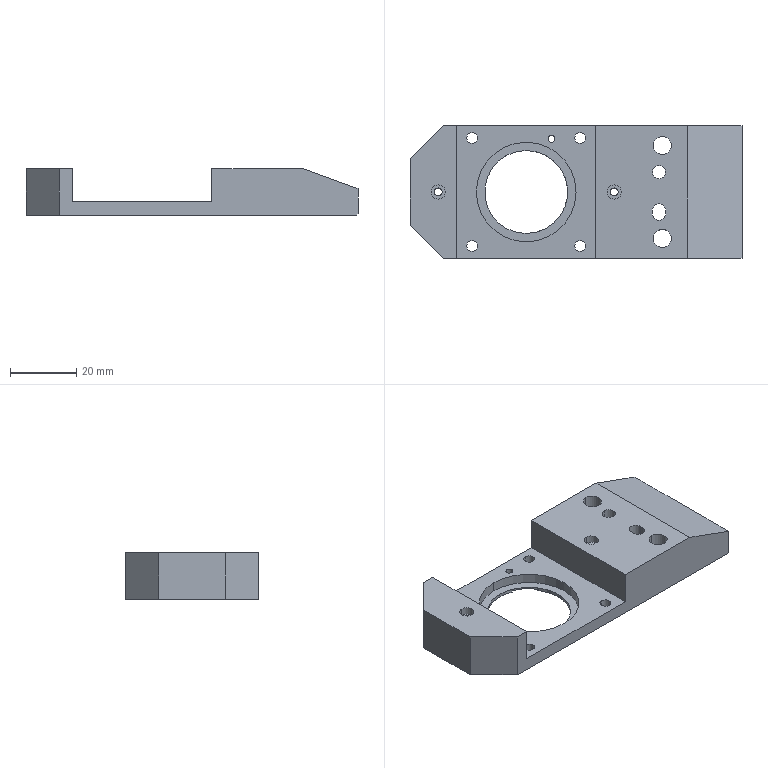NC program | NX | posted with a generic post | part box 100 x 40 x 14 mm
Lines 8469 to 9279 of 15435:
(HOLE_MILLING , TOOL : D3)
N16852 T17 M6
N16854 G54
N16856 G17 G0 G90 X-41.5 Y0. S5500 M3
N16858 G43 Z30. H17
N16860 Z0.5
N16862 G94 G3 X-41.175 Y-0.325 R0.325 F1250.
N16864 X-40.85 Y0. R0.325
N16866 X-40.85 Y0. Z0.44 I-0.65 J0.
N16868 X-40.85 Y0. Z0.38 I-0.65 J0.
N16870 X-40.85 Y0. Z0.32 I-0.65 J0.
N16872 X-40.85 Y0. Z0.26 I-0.65 J0.
N16874 X-40.85 Y0. Z0.2 I-0.65 J0.
N16876 X-40.85 Y0. Z0.14 I-0.65 J0.
N16878 X-40.85 Y0. Z0.08 I-0.65 J0.
N16880 X-40.85 Y0. Z0.02 I-0.65 J0.
N16882 X-40.85 Y0. Z-0.04 I-0.65 J0.
N16884 X-40.85 Y0. Z-0.1 I-0.65 J0.
N16886 X-40.85 Y0. Z-0.16 I-0.65 J0.
N16888 X-40.85 Y0. Z-0.22 I-0.65 J0.
N16890 X-40.85 Y0. Z-0.28 I-0.65 J0.
N16892 X-40.85 Y0. Z-0.34 I-0.65 J0.
N16894 X-40.85 Y0. Z-0.4 I-0.65 J0.
N16896 X-40.85 Y0. Z-0.46 I-0.65 J0.
N16898 X-40.85 Y0. Z-0.52 I-0.65 J0.
N16900 X-40.85 Y0. Z-0.58 I-0.65 J0.
N16902 X-40.85 Y0. Z-0.64 I-0.65 J0.
N16904 X-40.85 Y0. Z-0.7 I-0.65 J0.
N16906 X-40.85 Y0. Z-0.76 I-0.65 J0.
N16908 X-40.85 Y0. Z-0.82 I-0.65 J0.
N16910 X-40.85 Y0. Z-0.88 I-0.65 J0.
N16912 X-40.85 Y0. Z-0.94 I-0.65 J0.
N16914 X-40.85 Y0. Z-1. I-0.65 J0.
N16916 X-40.85 Y0. Z-1.06 I-0.65 J0.
N16918 X-40.85 Y0. Z-1.12 I-0.65 J0.
N16920 X-40.85 Y0. Z-1.18 I-0.65 J0.
N16922 X-40.85 Y0. Z-1.24 I-0.65 J0.
N16924 X-40.85 Y0. Z-1.3 I-0.65 J0.
N16926 X-40.85 Y0. Z-1.36 I-0.65 J0.
N16928 X-40.85 Y0. Z-1.42 I-0.65 J0.
N16930 X-40.85 Y0. Z-1.48 I-0.65 J0.
N16932 X-40.85 Y0. Z-1.54 I-0.65 J0.
N16934 X-40.85 Y0. Z-1.6 I-0.65 J0.
N16936 X-40.85 Y0. Z-1.66 I-0.65 J0.
N16938 X-40.85 Y0. Z-1.72 I-0.65 J0.
N16940 X-40.85 Y0. Z-1.78 I-0.65 J0.
N16942 X-40.85 Y0. Z-1.84 I-0.65 J0.
N16944 X-40.85 Y0. Z-1.9 I-0.65 J0.
N16946 X-40.85 Y0. Z-1.96 I-0.65 J0.
N16948 X-40.85 Y0. Z-2.02 I-0.65 J0.
N16950 X-40.85 Y0. Z-2.08 I-0.65 J0.
N16952 X-40.85 Y0. Z-2.14 I-0.65 J0.
N16954 X-40.85 Y0. Z-2.2 I-0.65 J0.
N16956 X-40.85 Y0. Z-2.26 I-0.65 J0.
N16958 X-41.825 Y-0.563 Z-2.3 R-0.65
N16960 X-40.937 Y-0.325 R0.65
N16962 X-41.825 Y-0.563 R-0.65
N16964 X-41.381 Y-0.444 R0.325
N16966 X-41.5 Y0. R0.325
N16968 G0 Z30.
N16970 X11.5
N16972 Z0.5
N16974 G3 X11.825 Y-0.325 R0.325
N16976 X12.15 Y0. R0.325
N16978 X12.15 Y0. Z0.44 I-0.65 J0.
N16980 X12.15 Y0. Z0.38 I-0.65 J0.
N16982 X12.15 Y0. Z0.32 I-0.65 J0.
N16984 X12.15 Y0. Z0.26 I-0.65 J0.
N16986 X12.15 Y0. Z0.2 I-0.65 J0.
N16988 X12.15 Y0. Z0.14 I-0.65 J0.
N16990 X12.15 Y0. Z0.08 I-0.65 J0.
N16992 X12.15 Y0. Z0.02 I-0.65 J0.
N16994 X12.15 Y0. Z-0.04 I-0.65 J0.
N16996 X12.15 Y0. Z-0.1 I-0.65 J0.
N16998 X12.15 Y0. Z-0.16 I-0.65 J0.
N17000 X12.15 Y0. Z-0.22 I-0.65 J0.
N17002 X12.15 Y0. Z-0.28 I-0.65 J0.
N17004 X12.15 Y0. Z-0.34 I-0.65 J0.
N17006 X12.15 Y0. Z-0.4 I-0.65 J0.
N17008 X12.15 Y0. Z-0.46 I-0.65 J0.
N17010 X12.15 Y0. Z-0.52 I-0.65 J0.
N17012 X12.15 Y0. Z-0.58 I-0.65 J0.
N17014 X12.15 Y0. Z-0.64 I-0.65 J0.
N17016 X12.15 Y0. Z-0.7 I-0.65 J0.
N17018 X12.15 Y0. Z-0.76 I-0.65 J0.
N17020 X12.15 Y0. Z-0.82 I-0.65 J0.
N17022 X12.15 Y0. Z-0.88 I-0.65 J0.
N17024 X12.15 Y0. Z-0.94 I-0.65 J0.
N17026 X12.15 Y0. Z-1. I-0.65 J0.
N17028 X12.15 Y0. Z-1.06 I-0.65 J0.
N17030 X12.15 Y0. Z-1.12 I-0.65 J0.
N17032 X12.15 Y0. Z-1.18 I-0.65 J0.
N17034 X12.15 Y0. Z-1.24 I-0.65 J0.
N17036 X12.15 Y0. Z-1.3 I-0.65 J0.
N17038 X12.15 Y0. Z-1.36 I-0.65 J0.
N17040 X12.15 Y0. Z-1.42 I-0.65 J0.
N17042 X12.15 Y0. Z-1.48 I-0.65 J0.
N17044 X12.15 Y0. Z-1.54 I-0.65 J0.
N17046 X12.15 Y0. Z-1.6 I-0.65 J0.
N17048 X12.15 Y0. Z-1.66 I-0.65 J0.
N17050 X12.15 Y0. Z-1.72 I-0.65 J0.
N17052 X12.15 Y0. Z-1.78 I-0.65 J0.
N17054 X12.15 Y0. Z-1.84 I-0.65 J0.
N17056 X12.15 Y0. Z-1.9 I-0.65 J0.
N17058 X12.15 Y0. Z-1.96 I-0.65 J0.
N17060 X12.15 Y0. Z-2.02 I-0.65 J0.
N17062 X12.15 Y0. Z-2.08 I-0.65 J0.
N17064 X12.15 Y0. Z-2.14 I-0.65 J0.
N17066 X12.15 Y0. Z-2.2 I-0.65 J0.
N17068 X12.15 Y0. Z-2.26 I-0.65 J0.
N17070 X11.175 Y-0.563 Z-2.3 R-0.65
N17072 X12.063 Y-0.325 R0.65
N17074 X11.175 Y-0.563 R-0.65
N17076 X11.619 Y-0.444 R0.325
N17078 X11.5 Y0. R0.325
N17080 G0 Z30.
(ZLEVEL_PROFILE_COPY_COPY_COPY , TOOL : D3)
N17082 X25.068 Y-5.056 S4500
N17084 Z1.
N17086 G1 X24.882 Z0.99 F1000.
N17088 X24.676 Y-5.173 Z0.978
N17090 X24.571 Y-5.333 Z0.968
N17092 X24.55 Y-5.405 Z0.964
N17094 Y-6.595 Z0.901
N17096 X24.676 Y-6.827 Z0.888
N17098 X24.908 Y-6.951 Z0.874
N17100 X25.099 Y-6.949 Z0.864
N17102 X25.327 Y-6.824 Z0.85
N17104 X25.45 Y-6.595 Z0.837
N17106 Y-5.405 Z0.774
N17108 X25.429 Y-5.333 Z0.77
N17110 X25.324 Y-5.173 Z0.76
N17112 X25.118 Y-5.056 Z0.748
N17114 X24.882 Z0.736
N17116 X24.676 Y-5.173 Z0.723
N17118 X24.571 Y-5.333 Z0.713
N17120 X24.55 Y-5.405 Z0.709
N17122 Y-6.595 Z0.647
N17124 X24.676 Y-6.827 Z0.633
N17126 X24.908 Y-6.951 Z0.619
N17128 X25.099 Y-6.949 Z0.609
N17130 X25.327 Y-6.824 Z0.596
N17132 X25.45 Y-6.595 Z0.582
N17134 Y-5.405 Z0.52
N17136 X25.429 Y-5.333 Z0.516
N17138 X25.324 Y-5.173 Z0.506
N17140 X25.118 Y-5.056 Z0.493
N17142 X24.882 Z0.481
N17144 X24.676 Y-5.173 Z0.468
N17146 X24.571 Y-5.333 Z0.458
N17148 X24.55 Y-5.405 Z0.454
N17150 Y-6.595 Z0.392
N17152 X24.676 Y-6.827 Z0.378
N17154 X24.908 Y-6.951 Z0.364
N17156 X25.099 Y-6.949 Z0.354
N17158 X25.327 Y-6.824 Z0.341
N17160 X25.45 Y-6.595 Z0.327
N17162 Y-5.405 Z0.265
N17164 X25.429 Y-5.333 Z0.261
N17166 X25.324 Y-5.173 Z0.251
N17168 X25.118 Y-5.056 Z0.238
N17170 X24.882 Z0.226
N17172 X24.676 Y-5.173 Z0.214
N17174 X24.571 Y-5.333 Z0.204
N17176 X24.55 Y-5.405 Z0.2
N17178 Y-6.595 Z0.137
N17180 X24.676 Y-6.827 Z0.124
N17182 X24.908 Y-6.951 Z0.11
N17184 X25.099 Y-6.949 Z0.1
N17186 X25.327 Y-6.824 Z0.086
N17188 X25.45 Y-6.595 Z0.072
N17190 Y-5.405 Z0.01
N17192 X25.429 Y-5.333 Z0.006
N17194 X25.324 Y-5.173 Z-0.004
N17196 X25.118 Y-5.056 Z-0.016
N17198 X24.882 Z-0.029
N17200 X24.676 Y-5.173 Z-0.041
N17202 X24.571 Y-5.333 Z-0.051
N17204 X24.55 Y-5.405 Z-0.055
N17206 Y-5.5 Z-0.06
N17208 Y-6.5 F1200.
N17210 G3 X25. Y-6.95 R0.45
N17212 X25.45 Y-6.5 R0.45
N17214 G1 Y-5.5
N17216 G3 X25. Y-5.05 R0.45
N17218 X24.55 Y-5.5 R0.45
N17220 G1 Y-6.482 Z-0.077
N17222 X24.565 Y-6.588 Z-0.079
N17224 X24.577 Y-6.639 Z-0.08
N17226 X24.588 Y-6.665
N17228 X24.613 Y-6.714 Z-0.081
N17230 X24.674 Y-6.798 Z-0.083
N17232 X24.732 Y-6.851 Z-0.085
N17234 X24.781 Y-6.884 Z-0.086
N17236 X24.871 Y-6.923 Z-0.087
N17238 X24.918 Y-6.934 Z-0.088
N17240 X24.949 Y-6.938 Z-0.089
N17242 X25.012 Y-6.942 Z-0.09
N17244 X25.108 Y-6.929 Z-0.092
N17246 X25.153 Y-6.915 Z-0.093
N17248 X25.183 Y-6.903
N17250 X25.239 Y-6.872 Z-0.094
N17252 X25.317 Y-6.811 Z-0.096
N17254 X25.366 Y-6.749 Z-0.097
N17256 X25.398 Y-6.694 Z-0.099
N17258 X25.421 Y-6.633 Z-0.1
N17260 X25.431 Y-6.602
N17262 X25.437 Y-6.554 Z-0.101
N17264 X25.448 Y-6.458 Z-0.103
N17266 X25.45 Y-6.336 Z-0.105
N17268 Y-5.722 Z-0.116
N17270 Y-5.599 Z-0.118
N17272 X25.449 Y-5.476 Z-0.12
N17274 G3 X24.55 Y-5.5 R0.45
N17276 G1 Y-6.482 Z-0.137
N17278 X24.565 Y-6.588 Z-0.139
N17280 X24.577 Y-6.639 Z-0.14
N17282 X24.588 Y-6.665
N17284 X24.613 Y-6.714 Z-0.141
N17286 X24.674 Y-6.798 Z-0.143
N17288 X24.732 Y-6.851 Z-0.145
N17290 X24.781 Y-6.884 Z-0.146
N17292 X24.871 Y-6.923 Z-0.147
N17294 X24.918 Y-6.934 Z-0.148
N17296 X24.949 Y-6.938 Z-0.149
N17298 X25.012 Y-6.942 Z-0.15
N17300 X25.108 Y-6.929 Z-0.152
N17302 X25.153 Y-6.915 Z-0.153
N17304 X25.183 Y-6.903
N17306 X25.239 Y-6.872 Z-0.154
N17308 X25.317 Y-6.811 Z-0.156
N17310 X25.366 Y-6.749 Z-0.157
N17312 X25.398 Y-6.694 Z-0.159
N17314 X25.421 Y-6.633 Z-0.16
N17316 X25.431 Y-6.602
N17318 X25.437 Y-6.554 Z-0.161
N17320 X25.448 Y-6.458 Z-0.163
N17322 X25.45 Y-6.336 Z-0.165
N17324 Y-5.722 Z-0.176
N17326 Y-5.599 Z-0.178
N17328 X25.449 Y-5.476 Z-0.18
N17330 G3 X24.55 Y-5.5 R0.45
N17332 G1 Y-6.482 Z-0.197
N17334 X24.565 Y-6.588 Z-0.199
N17336 X24.577 Y-6.639 Z-0.2
N17338 X24.588 Y-6.665
N17340 X24.613 Y-6.714 Z-0.201
N17342 X24.674 Y-6.798 Z-0.203
N17344 X24.732 Y-6.851 Z-0.205
N17346 X24.781 Y-6.884 Z-0.206
N17348 X24.871 Y-6.923 Z-0.207
N17350 X24.918 Y-6.934 Z-0.208
N17352 X24.949 Y-6.938 Z-0.209
N17354 X25.012 Y-6.942 Z-0.21
N17356 X25.108 Y-6.929 Z-0.212
N17358 X25.153 Y-6.915 Z-0.213
N17360 X25.183 Y-6.903
N17362 X25.239 Y-6.872 Z-0.214
N17364 X25.317 Y-6.811 Z-0.216
N17366 X25.366 Y-6.749 Z-0.217
N17368 X25.398 Y-6.694 Z-0.219
N17370 X25.421 Y-6.633 Z-0.22
N17372 X25.431 Y-6.602
N17374 X25.437 Y-6.554 Z-0.221
N17376 X25.448 Y-6.458 Z-0.223
N17378 X25.45 Y-6.336 Z-0.225
N17380 Y-5.722 Z-0.236
N17382 Y-5.599 Z-0.238
N17384 X25.449 Y-5.476 Z-0.24
N17386 G3 X24.55 Y-5.5 R0.45
N17388 G1 Y-6.482 Z-0.257
N17390 X24.565 Y-6.588 Z-0.259
N17392 X24.577 Y-6.639 Z-0.26
N17394 X24.588 Y-6.665
N17396 X24.613 Y-6.714 Z-0.261
N17398 X24.674 Y-6.798 Z-0.263
N17400 X24.732 Y-6.851 Z-0.265
N17402 X24.781 Y-6.884 Z-0.266
N17404 X24.871 Y-6.923 Z-0.267
N17406 X24.918 Y-6.934 Z-0.268
N17408 X24.949 Y-6.938 Z-0.269
N17410 X25.012 Y-6.942 Z-0.27
N17412 X25.108 Y-6.929 Z-0.272
N17414 X25.153 Y-6.915 Z-0.273
N17416 X25.183 Y-6.903
N17418 X25.239 Y-6.872 Z-0.274
N17420 X25.317 Y-6.811 Z-0.276
N17422 X25.366 Y-6.749 Z-0.277
N17424 X25.398 Y-6.694 Z-0.279
N17426 X25.421 Y-6.633 Z-0.28
N17428 X25.431 Y-6.602
N17430 X25.437 Y-6.554 Z-0.281
N17432 X25.448 Y-6.458 Z-0.283
N17434 X25.45 Y-6.336 Z-0.285
N17436 Y-5.722 Z-0.296
N17438 Y-5.599 Z-0.298
N17440 X25.449 Y-5.476 Z-0.3
N17442 G3 X24.55 Y-5.5 R0.45
N17444 G1 Y-6.482 Z-0.317
N17446 X24.565 Y-6.588 Z-0.319
N17448 X24.577 Y-6.639 Z-0.32
N17450 X24.588 Y-6.665
N17452 X24.613 Y-6.714 Z-0.321
N17454 X24.674 Y-6.798 Z-0.323
N17456 X24.732 Y-6.851 Z-0.325
N17458 X24.781 Y-6.884 Z-0.326
N17460 X24.871 Y-6.923 Z-0.327
N17462 X24.918 Y-6.934 Z-0.328
N17464 X24.949 Y-6.938 Z-0.329
N17466 X25.012 Y-6.942 Z-0.33
N17468 X25.108 Y-6.929 Z-0.332
N17470 X25.153 Y-6.915 Z-0.333
N17472 X25.183 Y-6.903
N17474 X25.239 Y-6.872 Z-0.334
N17476 X25.317 Y-6.811 Z-0.336
N17478 X25.366 Y-6.749 Z-0.337
N17480 X25.398 Y-6.694 Z-0.339
N17482 X25.421 Y-6.633 Z-0.34
N17484 X25.431 Y-6.602
N17486 X25.437 Y-6.554 Z-0.341
N17488 X25.448 Y-6.458 Z-0.343
N17490 X25.45 Y-6.336 Z-0.345
N17492 Y-5.722 Z-0.356
N17494 Y-5.599 Z-0.358
N17496 X25.449 Y-5.476 Z-0.36
N17498 G3 X24.55 Y-5.5 R0.45
N17500 G1 Y-6.482 Z-0.377
N17502 X24.565 Y-6.588 Z-0.379
N17504 X24.577 Y-6.639 Z-0.38
N17506 X24.588 Y-6.665
N17508 X24.613 Y-6.714 Z-0.381
N17510 X24.674 Y-6.798 Z-0.383
N17512 X24.709 Y-6.833 Z-0.384
N17514 X24.732 Y-6.851 Z-0.385
N17516 X24.781 Y-6.884 Z-0.386
N17518 X24.871 Y-6.923 Z-0.387
N17520 X24.918 Y-6.934 Z-0.388
N17522 X24.949 Y-6.938 Z-0.389
N17524 X25.012 Y-6.942 Z-0.39
N17526 X25.108 Y-6.929 Z-0.392
N17528 X25.153 Y-6.915 Z-0.393
N17530 X25.183 Y-6.903
N17532 X25.239 Y-6.872 Z-0.394
N17534 X25.317 Y-6.811 Z-0.396
N17536 X25.366 Y-6.749 Z-0.397
N17538 X25.398 Y-6.694 Z-0.399
N17540 X25.421 Y-6.633 Z-0.4
N17542 X25.431 Y-6.602
N17544 X25.437 Y-6.554 Z-0.401
N17546 X25.448 Y-6.458 Z-0.403
N17548 X25.45 Y-6.336 Z-0.405
N17550 Y-5.722 Z-0.416
N17552 Y-5.599 Z-0.418
N17554 X25.449 Y-5.476 Z-0.42
N17556 G3 X24.55 Y-5.5 R0.45
N17558 G1 Y-6.482 Z-0.437
N17560 X24.565 Y-6.588 Z-0.439
N17562 X24.577 Y-6.639 Z-0.44
N17564 X24.588 Y-6.665
N17566 X24.613 Y-6.714 Z-0.441
N17568 X24.674 Y-6.798 Z-0.443
N17570 X24.709 Y-6.833 Z-0.444
N17572 X24.732 Y-6.851 Z-0.445
N17574 X24.781 Y-6.884 Z-0.446
N17576 X24.871 Y-6.923 Z-0.447
N17578 X24.918 Y-6.934 Z-0.448
N17580 X24.949 Y-6.938 Z-0.449
N17582 X25.012 Y-6.942 Z-0.45
N17584 X25.108 Y-6.929 Z-0.452
N17586 X25.153 Y-6.915 Z-0.453
N17588 X25.183 Y-6.903
N17590 X25.239 Y-6.872 Z-0.454
N17592 X25.317 Y-6.811 Z-0.456
N17594 X25.366 Y-6.749 Z-0.457
N17596 X25.398 Y-6.694 Z-0.459
N17598 X25.421 Y-6.633 Z-0.46
N17600 X25.431 Y-6.602
N17602 X25.437 Y-6.554 Z-0.461
N17604 X25.448 Y-6.458 Z-0.463
N17606 X25.45 Y-6.336 Z-0.465
N17608 Y-5.722 Z-0.476
N17610 Y-5.599 Z-0.478
N17612 X25.449 Y-5.476 Z-0.48
N17614 G3 X24.55 Y-5.5 R0.45
N17616 G1 Y-6.482 Z-0.497
N17618 X24.565 Y-6.588 Z-0.499
N17620 X24.577 Y-6.639 Z-0.5
N17622 X24.588 Y-6.665
N17624 X24.613 Y-6.714 Z-0.501
N17626 X24.674 Y-6.798 Z-0.503
N17628 X24.709 Y-6.833 Z-0.504
N17630 X24.732 Y-6.851 Z-0.505
N17632 X24.781 Y-6.884 Z-0.506
N17634 X24.871 Y-6.923 Z-0.507
N17636 X24.918 Y-6.934 Z-0.508
N17638 X24.949 Y-6.938 Z-0.509
N17640 X25.012 Y-6.942 Z-0.51
N17642 X25.108 Y-6.929 Z-0.512
N17644 X25.153 Y-6.915 Z-0.513
N17646 X25.183 Y-6.903
N17648 X25.239 Y-6.872 Z-0.514
N17650 X25.317 Y-6.811 Z-0.516
N17652 X25.366 Y-6.749 Z-0.517
N17654 X25.398 Y-6.694 Z-0.519
N17656 X25.421 Y-6.633 Z-0.52
N17658 X25.431 Y-6.602
N17660 X25.437 Y-6.554 Z-0.521
N17662 X25.448 Y-6.458 Z-0.523
N17664 X25.45 Y-6.336 Z-0.525
N17666 Y-5.722 Z-0.536
N17668 Y-5.599 Z-0.538
N17670 X25.449 Y-5.476 Z-0.54
N17672 G3 X24.55 Y-5.5 R0.45
N17674 G1 Y-6.482 Z-0.557
N17676 X24.565 Y-6.588 Z-0.559
N17678 X24.577 Y-6.639 Z-0.56
N17680 X24.588 Y-6.665
N17682 X24.613 Y-6.714 Z-0.561
N17684 X24.674 Y-6.798 Z-0.563
N17686 X24.709 Y-6.833 Z-0.564
N17688 X24.732 Y-6.851 Z-0.565
N17690 X24.781 Y-6.884 Z-0.566
N17692 X24.871 Y-6.923 Z-0.567
N17694 X24.918 Y-6.934 Z-0.568
N17696 X24.949 Y-6.938 Z-0.569
N17698 X25.012 Y-6.942 Z-0.57
N17700 X25.108 Y-6.929 Z-0.572
N17702 X25.153 Y-6.915 Z-0.573
N17704 X25.183 Y-6.903
N17706 X25.239 Y-6.872 Z-0.574
N17708 X25.317 Y-6.811 Z-0.576
N17710 X25.366 Y-6.749 Z-0.577
N17712 X25.398 Y-6.694 Z-0.579
N17714 X25.421 Y-6.633 Z-0.58
N17716 X25.431 Y-6.602
N17718 X25.437 Y-6.554 Z-0.581
N17720 X25.448 Y-6.458 Z-0.583
N17722 X25.45 Y-6.336 Z-0.585
N17724 Y-5.722 Z-0.596
N17726 Y-5.599 Z-0.598
N17728 X25.449 Y-5.476 Z-0.6
N17730 G3 X24.55 Y-5.5 R0.45
N17732 G1 Y-6.482 Z-0.617
N17734 X24.565 Y-6.588 Z-0.619
N17736 X24.577 Y-6.639 Z-0.62
N17738 X24.588 Y-6.665
N17740 X24.613 Y-6.714 Z-0.621
N17742 X24.674 Y-6.798 Z-0.623
N17744 X24.709 Y-6.833 Z-0.624
N17746 X24.732 Y-6.851 Z-0.625
N17748 X24.781 Y-6.884 Z-0.626
N17750 X24.871 Y-6.923 Z-0.627
N17752 X24.918 Y-6.934 Z-0.628
N17754 X24.949 Y-6.938 Z-0.629
N17756 X25.012 Y-6.942 Z-0.63
N17758 X25.108 Y-6.929 Z-0.632
N17760 X25.153 Y-6.915 Z-0.633
N17762 X25.183 Y-6.903
N17764 X25.239 Y-6.872 Z-0.634
N17766 X25.317 Y-6.811 Z-0.636
N17768 X25.366 Y-6.749 Z-0.637
N17770 X25.398 Y-6.694 Z-0.639
N17772 X25.421 Y-6.633 Z-0.64
N17774 X25.431 Y-6.602
N17776 X25.437 Y-6.554 Z-0.641
N17778 X25.448 Y-6.458 Z-0.643
N17780 X25.45 Y-6.336 Z-0.645
N17782 Y-5.722 Z-0.656
N17784 Y-5.599 Z-0.658
N17786 X25.449 Y-5.476 Z-0.66
N17788 G3 X24.55 Y-5.5 R0.45
N17790 G1 Y-6.482 Z-0.677
N17792 X24.565 Y-6.588 Z-0.679
N17794 X24.577 Y-6.639 Z-0.68
N17796 X24.588 Y-6.665
N17798 X24.613 Y-6.714 Z-0.681
N17800 X24.674 Y-6.798 Z-0.683
N17802 X24.709 Y-6.833 Z-0.684
N17804 X24.732 Y-6.851 Z-0.685
N17806 X24.781 Y-6.884 Z-0.686
N17808 X24.871 Y-6.923 Z-0.687
N17810 X24.918 Y-6.934 Z-0.688
N17812 X24.949 Y-6.938 Z-0.689
N17814 X25.012 Y-6.942 Z-0.69
N17816 X25.108 Y-6.929 Z-0.692
N17818 X25.153 Y-6.915 Z-0.693
N17820 X25.183 Y-6.903
N17822 X25.239 Y-6.872 Z-0.694
N17824 X25.317 Y-6.811 Z-0.696
N17826 X25.366 Y-6.749 Z-0.697
N17828 X25.398 Y-6.694 Z-0.699
N17830 X25.421 Y-6.633 Z-0.7
N17832 X25.431 Y-6.602
N17834 X25.437 Y-6.554 Z-0.701
N17836 X25.448 Y-6.458 Z-0.703
N17838 X25.45 Y-6.336 Z-0.705
N17840 Y-5.722 Z-0.716
N17842 Y-5.599 Z-0.718
N17844 X25.449 Y-5.476 Z-0.72
N17846 G3 X24.55 Y-5.5 R0.45
N17848 G1 Y-6.482 Z-0.737
N17850 X24.565 Y-6.588 Z-0.739
N17852 X24.577 Y-6.639 Z-0.74
N17854 X24.588 Y-6.665
N17856 X24.613 Y-6.714 Z-0.741
N17858 X24.674 Y-6.798 Z-0.743
N17860 X24.709 Y-6.833 Z-0.744
N17862 X24.732 Y-6.851 Z-0.745
N17864 X24.781 Y-6.884 Z-0.746
N17866 X24.871 Y-6.923 Z-0.747
N17868 X24.918 Y-6.934 Z-0.748
N17870 X24.949 Y-6.938 Z-0.749
N17872 X25.012 Y-6.942 Z-0.75
N17874 X25.108 Y-6.929 Z-0.752
N17876 X25.153 Y-6.915 Z-0.753
N17878 X25.183 Y-6.903
N17880 X25.239 Y-6.872 Z-0.754
N17882 X25.317 Y-6.811 Z-0.756
N17884 X25.366 Y-6.749 Z-0.757
N17886 X25.398 Y-6.694 Z-0.759
N17888 X25.421 Y-6.633 Z-0.76
N17890 X25.431 Y-6.602
N17892 X25.437 Y-6.554 Z-0.761
N17894 X25.448 Y-6.458 Z-0.763
N17896 X25.45 Y-6.336 Z-0.765
N17898 Y-5.722 Z-0.776
N17900 Y-5.599 Z-0.778
N17902 X25.449 Y-5.476 Z-0.78
N17904 G3 X24.55 Y-5.5 R0.45
N17906 G1 Y-6.482 Z-0.797
N17908 X24.565 Y-6.588 Z-0.799
N17910 X24.577 Y-6.639 Z-0.8
N17912 X24.588 Y-6.665
N17914 X24.613 Y-6.714 Z-0.801
N17916 X24.674 Y-6.798 Z-0.803
N17918 X24.709 Y-6.833 Z-0.804
N17920 X24.732 Y-6.851 Z-0.805
N17922 X24.781 Y-6.884 Z-0.806
N17924 X24.871 Y-6.923 Z-0.807
N17926 X24.918 Y-6.934 Z-0.808
N17928 X24.949 Y-6.938 Z-0.809
N17930 X25.012 Y-6.942 Z-0.81
N17932 X25.108 Y-6.929 Z-0.812
N17934 X25.153 Y-6.915 Z-0.813
N17936 X25.183 Y-6.903
N17938 X25.239 Y-6.872 Z-0.814
N17940 X25.317 Y-6.811 Z-0.816
N17942 X25.366 Y-6.749 Z-0.817
N17944 X25.398 Y-6.694 Z-0.819
N17946 X25.421 Y-6.633 Z-0.82
N17948 X25.431 Y-6.602
N17950 X25.437 Y-6.554 Z-0.821
N17952 X25.448 Y-6.458 Z-0.823
N17954 X25.45 Y-6.336 Z-0.825
N17956 Y-5.722 Z-0.836
N17958 Y-5.599 Z-0.838
N17960 X25.449 Y-5.476 Z-0.84
N17962 G3 X24.55 Y-5.5 R0.45
N17964 G1 Y-6.482 Z-0.857
N17966 X24.565 Y-6.588 Z-0.859
N17968 X24.577 Y-6.639 Z-0.86
N17970 X24.588 Y-6.665
N17972 X24.613 Y-6.714 Z-0.861
N17974 X24.674 Y-6.798 Z-0.863
N17976 X24.709 Y-6.833 Z-0.864
N17978 X24.732 Y-6.851 Z-0.865
N17980 X24.781 Y-6.884 Z-0.866
N17982 X24.871 Y-6.923 Z-0.867
N17984 X24.917 Y-6.936 Z-0.868
N17986 X25.012 Y-6.942 Z-0.87
N17988 X25.108 Y-6.929 Z-0.872
N17990 X25.153 Y-6.915 Z-0.873
N17992 X25.183 Y-6.903
N17994 X25.239 Y-6.872 Z-0.874
N17996 X25.317 Y-6.811 Z-0.876
N17998 X25.366 Y-6.749 Z-0.877
N18000 X25.398 Y-6.694 Z-0.879
N18002 X25.421 Y-6.633 Z-0.88
N18004 X25.431 Y-6.602
N18006 X25.437 Y-6.554 Z-0.881
N18008 X25.448 Y-6.458 Z-0.883
N18010 X25.45 Y-6.336 Z-0.885
N18012 Y-5.722 Z-0.896
N18014 Y-5.599 Z-0.898
N18016 X25.449 Y-5.476 Z-0.9
N18018 G3 X24.55 Y-5.5 R0.45
N18020 G1 Y-6.482 Z-0.917
N18022 X24.565 Y-6.588 Z-0.919
N18024 X24.577 Y-6.639 Z-0.92
N18026 X24.588 Y-6.665
N18028 X24.613 Y-6.714 Z-0.921
N18030 X24.674 Y-6.798 Z-0.923
N18032 X24.709 Y-6.833 Z-0.924
N18034 X24.732 Y-6.851 Z-0.925
N18036 X24.781 Y-6.884 Z-0.926
N18038 X24.871 Y-6.923 Z-0.927
N18040 X24.917 Y-6.936 Z-0.928
N18042 X25.012 Y-6.942 Z-0.93
N18044 X25.108 Y-6.929 Z-0.932
N18046 X25.153 Y-6.915 Z-0.933
N18048 X25.183 Y-6.903
N18050 X25.239 Y-6.872 Z-0.934
N18052 X25.317 Y-6.811 Z-0.936
N18054 X25.366 Y-6.749 Z-0.937
N18056 X25.398 Y-6.694 Z-0.939
N18058 X25.421 Y-6.633 Z-0.94
N18060 X25.431 Y-6.602
N18062 X25.437 Y-6.554 Z-0.941
N18064 X25.448 Y-6.458 Z-0.943
N18066 X25.45 Y-6.336 Z-0.945
N18068 Y-5.722 Z-0.956
N18070 Y-5.599 Z-0.958
N18072 X25.449 Y-5.476 Z-0.96
N18074 G3 X24.55 Y-5.5 R0.45
N18076 G1 Y-6.482 Z-0.977
N18078 X24.565 Y-6.588 Z-0.979
N18080 X24.577 Y-6.639 Z-0.98
N18082 X24.588 Y-6.665
N18084 X24.613 Y-6.714 Z-0.981
N18086 X24.674 Y-6.798 Z-0.983
N18088 X24.709 Y-6.833 Z-0.984
N18090 X24.732 Y-6.851 Z-0.985
N18092 X24.781 Y-6.884 Z-0.986
N18094 X24.871 Y-6.923 Z-0.987
N18096 X24.917 Y-6.936 Z-0.988
N18098 X25.012 Y-6.942 Z-0.99
N18100 X25.108 Y-6.929 Z-0.992
N18102 X25.153 Y-6.915 Z-0.993
N18104 X25.183 Y-6.903
N18106 X25.239 Y-6.872 Z-0.994
N18108 X25.317 Y-6.811 Z-0.996
N18110 X25.366 Y-6.749 Z-0.997
N18112 X25.398 Y-6.694 Z-0.999
N18114 X25.421 Y-6.633 Z-1.
N18116 X25.431 Y-6.602
N18118 X25.437 Y-6.554 Z-1.001
N18120 X25.448 Y-6.458 Z-1.003
N18122 X25.45 Y-6.336 Z-1.005
N18124 Y-5.722 Z-1.016
N18126 Y-5.599 Z-1.018
N18128 X25.449 Y-5.476 Z-1.02
N18130 G3 X24.55 Y-5.5 R0.45
N18132 G1 Y-6.482 Z-1.037
N18134 X24.565 Y-6.588 Z-1.039
N18136 X24.577 Y-6.639 Z-1.04
N18138 X24.588 Y-6.665
N18140 X24.613 Y-6.714 Z-1.041
N18142 X24.674 Y-6.797 Z-1.043
N18144 X24.709 Y-6.833 Z-1.044
N18146 X24.732 Y-6.851 Z-1.045
N18148 X24.781 Y-6.884 Z-1.046
N18150 X24.871 Y-6.923 Z-1.047
N18152 X24.917 Y-6.936 Z-1.048
N18154 X25.012 Y-6.942 Z-1.05
N18156 X25.108 Y-6.929 Z-1.052
N18158 X25.153 Y-6.915 Z-1.053
N18160 X25.183 Y-6.903
N18162 X25.239 Y-6.872 Z-1.054
N18164 X25.317 Y-6.811 Z-1.056
N18166 X25.366 Y-6.749 Z-1.057
N18168 X25.398 Y-6.694 Z-1.059
N18170 X25.421 Y-6.633 Z-1.06
N18172 X25.431 Y-6.602
N18174 X25.437 Y-6.554 Z-1.061
N18176 X25.448 Y-6.458 Z-1.063
N18178 X25.45 Y-6.336 Z-1.065
N18180 Y-5.722 Z-1.076
N18182 Y-5.599 Z-1.078
N18184 X25.449 Y-5.476 Z-1.08
N18186 G3 X24.55 Y-5.5 R0.45
N18188 G1 Y-6.482 Z-1.097
N18190 X24.565 Y-6.588 Z-1.099
N18192 X24.577 Y-6.639 Z-1.1
N18194 X24.588 Y-6.665
N18196 X24.613 Y-6.714 Z-1.101
N18198 X24.674 Y-6.797 Z-1.103
N18200 X24.709 Y-6.833 Z-1.104
N18202 X24.732 Y-6.851 Z-1.105
N18204 X24.781 Y-6.884 Z-1.106
N18206 X24.871 Y-6.923 Z-1.107
N18208 X24.917 Y-6.936 Z-1.108
N18210 X25.012 Y-6.942 Z-1.11
N18212 X25.108 Y-6.929 Z-1.112
N18214 X25.153 Y-6.915 Z-1.113
N18216 X25.183 Y-6.903
N18218 X25.239 Y-6.872 Z-1.114
N18220 X25.317 Y-6.811 Z-1.116
N18222 X25.366 Y-6.749 Z-1.117
N18224 X25.398 Y-6.694 Z-1.119
N18226 X25.421 Y-6.633 Z-1.12
N18228 X25.431 Y-6.602
N18230 X25.437 Y-6.554 Z-1.121
N18232 X25.448 Y-6.458 Z-1.123
N18234 X25.45 Y-6.336 Z-1.125
N18236 Y-5.722 Z-1.136
N18238 Y-5.599 Z-1.138
N18240 X25.449 Y-5.476 Z-1.14
N18242 G3 X24.55 Y-5.5 R0.45
N18244 G1 Y-6.482 Z-1.157
N18246 X24.565 Y-6.588 Z-1.159
N18248 X24.577 Y-6.639 Z-1.16
N18250 X24.588 Y-6.665
N18252 X24.613 Y-6.714 Z-1.161
N18254 X24.673 Y-6.797 Z-1.163
N18256 X24.709 Y-6.833 Z-1.164
N18258 X24.732 Y-6.851 Z-1.165
N18260 X24.781 Y-6.884 Z-1.166
N18262 X24.871 Y-6.923 Z-1.167
N18264 X24.917 Y-6.936 Z-1.168
N18266 X25.012 Y-6.942 Z-1.17
N18268 X25.108 Y-6.929 Z-1.172
N18270 X25.153 Y-6.915 Z-1.173
N18272 X25.183 Y-6.903
N18274 X25.239 Y-6.872 Z-1.174
N18276 X25.317 Y-6.811 Z-1.176
N18278 X25.366 Y-6.749 Z-1.177
N18280 X25.398 Y-6.694 Z-1.179
N18282 X25.421 Y-6.633 Z-1.18
N18284 X25.431 Y-6.602
N18286 X25.437 Y-6.554 Z-1.181
N18288 X25.448 Y-6.458 Z-1.183
N18290 X25.45 Y-6.336 Z-1.185
N18292 Y-5.722 Z-1.196
N18294 Y-5.599 Z-1.198
N18296 X25.449 Y-5.476 Z-1.2
N18298 G3 X24.55 Y-5.5 R0.45
N18300 G1 Y-6.482 Z-1.217
N18302 X24.565 Y-6.588 Z-1.219
N18304 X24.577 Y-6.639 Z-1.22
N18306 X24.588 Y-6.665
N18308 X24.613 Y-6.714 Z-1.221
N18310 X24.673 Y-6.797 Z-1.223
N18312 X24.709 Y-6.833 Z-1.224
N18314 X24.732 Y-6.851 Z-1.225
N18316 X24.781 Y-6.884 Z-1.226
N18318 X24.871 Y-6.923 Z-1.227
N18320 X24.917 Y-6.936 Z-1.228
N18322 X25.012 Y-6.942 Z-1.23
N18324 X25.108 Y-6.929 Z-1.232
N18326 X25.153 Y-6.915 Z-1.233
N18328 X25.183 Y-6.903
N18330 X25.239 Y-6.872 Z-1.234
N18332 X25.317 Y-6.811 Z-1.236
N18334 X25.366 Y-6.749 Z-1.237
N18336 X25.398 Y-6.694 Z-1.239
N18338 X25.421 Y-6.633 Z-1.24
N18340 X25.431 Y-6.602
N18342 X25.437 Y-6.554 Z-1.241
N18344 X25.448 Y-6.458 Z-1.243
N18346 X25.45 Y-6.336 Z-1.245
N18348 Y-5.722 Z-1.256
N18350 Y-5.599 Z-1.258
N18352 X25.449 Y-5.476 Z-1.26
N18354 G3 X24.55 Y-5.5 R0.45
N18356 G1 Y-6.482 Z-1.277
N18358 X24.565 Y-6.588 Z-1.279
N18360 X24.577 Y-6.639 Z-1.28
N18362 X24.588 Y-6.665
N18364 X24.613 Y-6.714 Z-1.281
N18366 X24.673 Y-6.797 Z-1.283
N18368 X24.709 Y-6.833 Z-1.284
N18370 X24.732 Y-6.851 Z-1.285
N18372 X24.781 Y-6.884 Z-1.286
N18374 X24.871 Y-6.923 Z-1.287
N18376 X24.917 Y-6.936 Z-1.288
N18378 X25.012 Y-6.942 Z-1.29
N18380 X25.108 Y-6.929 Z-1.292
N18382 X25.153 Y-6.915 Z-1.293
N18384 X25.183 Y-6.903
N18386 X25.239 Y-6.872 Z-1.294
N18388 X25.317 Y-6.811 Z-1.296
N18390 X25.366 Y-6.749 Z-1.297
N18392 X25.398 Y-6.694 Z-1.299
N18394 X25.421 Y-6.633 Z-1.3
N18396 X25.431 Y-6.602
N18398 X25.437 Y-6.554 Z-1.301
N18400 X25.448 Y-6.458 Z-1.303
N18402 X25.45 Y-6.336 Z-1.305
N18404 Y-5.722 Z-1.316
N18406 Y-5.599 Z-1.318
N18408 X25.449 Y-5.476 Z-1.32
N18410 G3 X24.55 Y-5.5 R0.45
N18412 G1 Y-6.482 Z-1.337
N18414 X24.565 Y-6.588 Z-1.339
N18416 X24.577 Y-6.639 Z-1.34
N18418 X24.588 Y-6.665
N18420 X24.613 Y-6.714 Z-1.341
N18422 X24.673 Y-6.797 Z-1.343
N18424 X24.709 Y-6.833 Z-1.344
N18426 X24.732 Y-6.851 Z-1.345
N18428 X24.781 Y-6.884 Z-1.346
N18430 X24.871 Y-6.923 Z-1.347
N18432 X24.917 Y-6.936 Z-1.348
N18434 X25.012 Y-6.942 Z-1.35
N18436 X25.108 Y-6.929 Z-1.352
N18438 X25.153 Y-6.915 Z-1.353
N18440 X25.183 Y-6.903
N18442 X25.239 Y-6.872 Z-1.354
N18444 X25.317 Y-6.811 Z-1.356
N18446 X25.366 Y-6.749 Z-1.357
N18448 X25.398 Y-6.694 Z-1.359
N18450 X25.421 Y-6.633 Z-1.36
N18452 X25.431 Y-6.602
N18454 X25.437 Y-6.554 Z-1.361
N18456 X25.448 Y-6.458 Z-1.363
N18458 X25.45 Y-6.336 Z-1.365
N18460 Y-5.722 Z-1.376